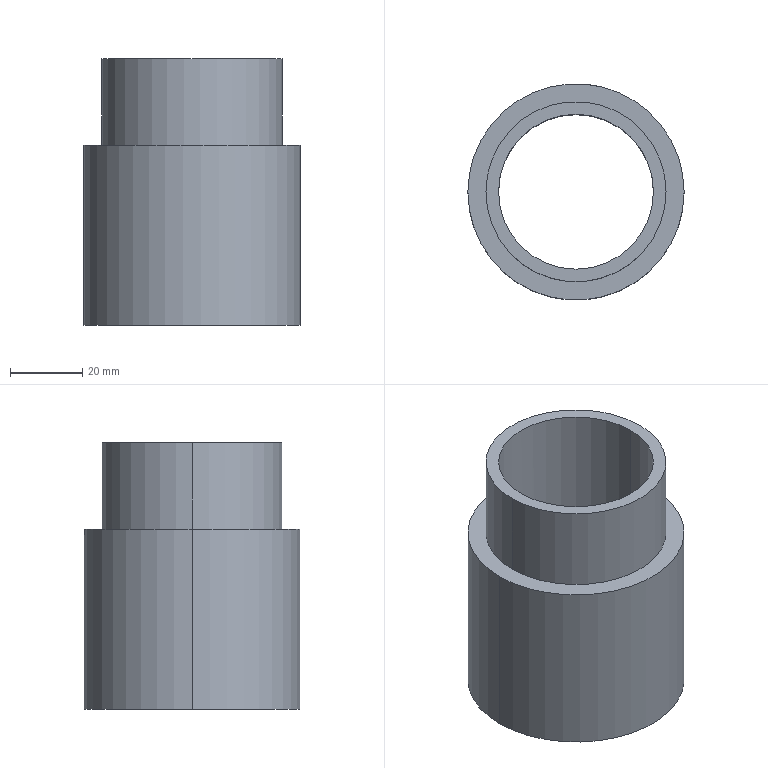Part | SolidWorks | features 3DProfileFeature 1, Extrusion 1, HoleWzd 1, ICE 1 | 1 solid | 11 faces | box 60 x 60 x 74 mm | volume 80866 mm3 | cylinder 8 | plane 3 | commonest cylinder face diameters 5 x2 43 x2 50 x2 60 x2
STEP:
#1=CARTESIAN_POINT('',(25.,0.,24.));
#2=VERTEX_POINT('',#1);
#3=CARTESIAN_POINT('',(-25.,0.,24.));
#4=VERTEX_POINT('',#3);
#5=CARTESIAN_POINT('',(0.,0.,24.));
#6=DIRECTION('',(0.,0.,1.));
#7=DIRECTION('',(1.,0.,0.));
#8=AXIS2_PLACEMENT_3D('',#5,#6,#7);
#9=CIRCLE('',#8,25.);
#10=EDGE_CURVE('',#2,#4,#9,.T.);
#11=ORIENTED_EDGE('',*,*,#10,.F.);
#12=CARTESIAN_POINT('',(25.,0.,0.));
#13=VERTEX_POINT('',#12);
#14=CARTESIAN_POINT('',(25.,0.,24.));
#15=DIRECTION('',(0.,0.,-1.));
#16=VECTOR('',#15,1000.);
#17=LINE('',#14,#16);
#18=EDGE_CURVE('',#2,#13,#17,.T.);
#19=ORIENTED_EDGE('',*,*,#18,.T.);
#20=CARTESIAN_POINT('',(-25.,0.,0.));
#21=VERTEX_POINT('',#20);
#22=CARTESIAN_POINT('',(0.,0.,0.));
#23=DIRECTION('',(0.,0.,1.));
#24=DIRECTION('',(1.,0.,0.));
#25=AXIS2_PLACEMENT_3D('',#22,#23,#24);
#26=CIRCLE('',#25,25.);
#27=EDGE_CURVE('',#13,#21,#26,.T.);
#28=ORIENTED_EDGE('',*,*,#27,.T.);
#29=CARTESIAN_POINT('',(-25.,0.,24.));
#30=DIRECTION('',(0.,0.,-1.));
#31=VECTOR('',#30,1000.);
#32=LINE('',#29,#31);
#33=EDGE_CURVE('',#4,#21,#32,.T.);
#34=ORIENTED_EDGE('',*,*,#33,.F.);
#35=EDGE_LOOP('',(#11,#19,#28,#34));
#36=FACE_OUTER_BOUND('',#35,.T.);
#37=CARTESIAN_POINT('',(0.,0.,24.));
#38=DIRECTION('',(0.,0.,-1.));
#39=DIRECTION('',(-1.,0.,0.));
#40=AXIS2_PLACEMENT_3D('',#37,#38,#39);
#41=CYLINDRICAL_SURFACE('',#40,25.);
#42=ADVANCED_FACE('',(#36),#41,.T.);
#43=CARTESIAN_POINT('',(4.954,20.921,-40.));
#44=VERTEX_POINT('',#43);
#45=CARTESIAN_POINT('',(-0.01248,21.5,-40.));
#46=VERTEX_POINT('',#45);
#47=CARTESIAN_POINT('',(4.954,20.921,-40.));
#48=CARTESIAN_POINT('',(4.954,20.921,-40.163));
#49=CARTESIAN_POINT('',(4.938,20.925,-40.325));
#50=CARTESIAN_POINT('',(4.876,20.94,-40.648));
#51=CARTESIAN_POINT('',(4.829,20.951,-40.806));
#52=CARTESIAN_POINT('',(4.706,20.979,-41.107));
#53=CARTESIAN_POINT('',(4.63,20.996,-41.252));
#54=CARTESIAN_POINT('',(4.451,21.034,-41.525));
#55=CARTESIAN_POINT('',(4.35,21.056,-41.651));
#56=CARTESIAN_POINT('',(4.123,21.101,-41.882));
#57=CARTESIAN_POINT('',(3.996,21.126,-41.987));
#58=CARTESIAN_POINT('',(3.729,21.175,-42.169));
#59=CARTESIAN_POINT('',(3.587,21.199,-42.246));
#60=CARTESIAN_POINT('',(3.288,21.248,-42.372));
#61=CARTESIAN_POINT('',(3.131,21.271,-42.42));
#62=CARTESIAN_POINT('',(2.815,21.316,-42.484));
#63=CARTESIAN_POINT('',(2.654,21.336,-42.5));
#64=CARTESIAN_POINT('',(2.325,21.375,-42.5));
#65=CARTESIAN_POINT('',(2.164,21.391,-42.484));
#66=CARTESIAN_POINT('',(1.845,21.421,-42.421));
#67=CARTESIAN_POINT('',(1.687,21.434,-42.373));
#68=CARTESIAN_POINT('',(1.384,21.456,-42.247));
#69=CARTESIAN_POINT('',(1.241,21.465,-42.171));
#70=CARTESIAN_POINT('',(0.9689,21.479,-41.989));
#71=CARTESIAN_POINT('',(0.8401,21.484,-41.884));
#72=CARTESIAN_POINT('',(0.6089,21.492,-41.654));
#73=CARTESIAN_POINT('',(0.505,21.494,-41.528));
#74=CARTESIAN_POINT('',(0.3212,21.498,-41.255));
#75=CARTESIAN_POINT('',(0.2431,21.499,-41.11));
#76=CARTESIAN_POINT('',(0.05455,21.5,-40.659));
#77=CARTESIAN_POINT('',(-0.01248,21.5,-40.331));
#78=CARTESIAN_POINT('',(-0.01248,21.5,-40.));
#79=B_SPLINE_CURVE_WITH_KNOTS('',3,(#47,#48,#49,#50,#51,#52,#53,#54,#55,#56,#57,#58,#59,#60,#61,#62,#63,#64,#65,#66,#67,#68,#69,#70,#71,#72,#73,#74,#75,#76,#77,#78),.UNSPECIFIED.,.F.,.F.,(4,2,2,2,2,2,2,2,2,2,2,2,2,2,2,4),(0.007823,0.008312,0.0088,0.009289,0.009778,0.01027,0.01076,0.01124,0.01173,0.01222,0.01271,0.0132,0.01369,0.01418,0.01467,0.01564),.UNSPECIFIED.);
#80=EDGE_CURVE('',#44,#46,#79,.T.);
#81=ORIENTED_EDGE('',*,*,#80,.F.);
#82=CARTESIAN_POINT('',(5.942,29.406,-40.));
#83=VERTEX_POINT('',#82);
#84=CARTESIAN_POINT('',(5.954,29.509,-40.));
#85=DIRECTION('',(0.1157,0.9933,0.));
#86=VECTOR('',#85,1000.);
#87=LINE('',#84,#86);
#88=EDGE_CURVE('',#44,#83,#87,.T.);
#89=ORIENTED_EDGE('',*,*,#88,.T.);
#90=CARTESIAN_POINT('',(0.9758,29.984,-40.));
#91=VERTEX_POINT('',#90);
#92=CARTESIAN_POINT('',(5.942,29.406,-40.));
#93=CARTESIAN_POINT('',(5.942,29.406,-40.163));
#94=CARTESIAN_POINT('',(5.927,29.409,-40.325));
#95=CARTESIAN_POINT('',(5.864,29.421,-40.648));
#96=CARTESIAN_POINT('',(5.816,29.431,-40.806));
#97=CARTESIAN_POINT('',(5.694,29.455,-41.107));
#98=CARTESIAN_POINT('',(5.618,29.469,-41.252));
#99=CARTESIAN_POINT('',(5.438,29.503,-41.525));
#100=CARTESIAN_POINT('',(5.336,29.522,-41.651));
#101=CARTESIAN_POINT('',(5.109,29.562,-41.882));
#102=CARTESIAN_POINT('',(4.982,29.584,-41.987));
#103=CARTESIAN_POINT('',(4.713,29.628,-42.169));
#104=CARTESIAN_POINT('',(4.572,29.65,-42.246));
#105=CARTESIAN_POINT('',(4.272,29.695,-42.372));
#106=CARTESIAN_POINT('',(4.115,29.717,-42.42));
#107=CARTESIAN_POINT('',(3.798,29.759,-42.484));
#108=CARTESIAN_POINT('',(3.637,29.779,-42.5));
#109=CARTESIAN_POINT('',(3.309,29.817,-42.5));
#110=CARTESIAN_POINT('',(3.147,29.835,-42.484));
#111=CARTESIAN_POINT('',(2.829,29.867,-42.421));
#112=CARTESIAN_POINT('',(2.671,29.881,-42.373));
#113=CARTESIAN_POINT('',(2.369,29.907,-42.247));
#114=CARTESIAN_POINT('',(2.226,29.918,-42.171));
#115=CARTESIAN_POINT('',(1.954,29.937,-41.99));
#116=CARTESIAN_POINT('',(1.826,29.945,-41.884));
#117=CARTESIAN_POINT('',(1.595,29.958,-41.654));
#118=CARTESIAN_POINT('',(1.491,29.963,-41.528));
#119=CARTESIAN_POINT('',(1.308,29.972,-41.255));
#120=CARTESIAN_POINT('',(1.23,29.975,-41.11));
#121=CARTESIAN_POINT('',(1.042,29.982,-40.659));
#122=CARTESIAN_POINT('',(0.9758,29.984,-40.33));
#123=CARTESIAN_POINT('',(0.9758,29.984,-40.));
#124=B_SPLINE_CURVE_WITH_KNOTS('',3,(#92,#93,#94,#95,#96,#97,#98,#99,#100,#101,#102,#103,#104,#105,#106,#107,#108,#109,#110,#111,#112,#113,#114,#115,#116,#117,#118,#119,#120,#121,#122,#123),.UNSPECIFIED.,.F.,.F.,(4,2,2,2,2,2,2,2,2,2,2,2,2,2,2,4),(0.00782,0.008308,0.008797,0.009285,0.009774,0.01026,0.01075,0.01124,0.01173,0.01222,0.01271,0.01319,0.01368,0.01417,0.01466,0.01564),.UNSPECIFIED.);
#125=EDGE_CURVE('',#83,#91,#124,.T.);
#126=ORIENTED_EDGE('',*,*,#125,.T.);
#127=CARTESIAN_POINT('',(0.9879,30.088,-40.));
#128=DIRECTION('',(0.1157,0.9933,0.));
#129=VECTOR('',#128,1000.);
#130=LINE('',#127,#129);
#131=EDGE_CURVE('',#46,#91,#130,.T.);
#132=ORIENTED_EDGE('',*,*,#131,.F.);
#133=EDGE_LOOP('',(#81,#89,#126,#132));
#134=FACE_OUTER_BOUND('',#133,.T.);
#135=CARTESIAN_POINT('',(3.471,29.799,-40.));
#136=DIRECTION('',(0.1157,0.9933,0.));
#137=DIRECTION('',(-0.9933,0.1157,0.));
#138=AXIS2_PLACEMENT_3D('',#135,#136,#137);
#139=CYLINDRICAL_SURFACE('',#138,2.5);
#140=ADVANCED_FACE('',(#134),#139,.F.);
#141=CARTESIAN_POINT('',(-21.5,0.,-50.));
#142=VERTEX_POINT('',#141);
#143=CARTESIAN_POINT('',(21.5,0.,-50.));
#144=VERTEX_POINT('',#143);
#145=CARTESIAN_POINT('',(0.,0.,-50.));
#146=DIRECTION('',(0.,0.,1.));
#147=DIRECTION('',(1.,0.,0.));
#148=AXIS2_PLACEMENT_3D('',#145,#146,#147);
#149=CIRCLE('',#148,21.5);
#150=EDGE_CURVE('',#142,#144,#149,.T.);
#151=ORIENTED_EDGE('',*,*,#150,.F.);
#152=CARTESIAN_POINT('',(-21.5,0.,24.));
#153=VERTEX_POINT('',#152);
#154=CARTESIAN_POINT('',(-21.5,0.,-50.));
#155=DIRECTION('',(0.,0.,1.));
#156=VECTOR('',#155,1000.);
#157=LINE('',#154,#156);
#158=EDGE_CURVE('',#142,#153,#157,.T.);
#159=ORIENTED_EDGE('',*,*,#158,.T.);
#160=CARTESIAN_POINT('',(21.5,0.,24.));
#161=VERTEX_POINT('',#160);
#162=CARTESIAN_POINT('',(0.,0.,24.));
#163=DIRECTION('',(0.,0.,1.));
#164=DIRECTION('',(1.,0.,0.));
#165=AXIS2_PLACEMENT_3D('',#162,#163,#164);
#166=CIRCLE('',#165,21.5);
#167=EDGE_CURVE('',#153,#161,#166,.T.);
#168=ORIENTED_EDGE('',*,*,#167,.T.);
#169=CARTESIAN_POINT('',(21.5,0.,-50.));
#170=DIRECTION('',(0.,0.,1.));
#171=VECTOR('',#170,1000.);
#172=LINE('',#169,#171);
#173=EDGE_CURVE('',#144,#161,#172,.T.);
#174=ORIENTED_EDGE('',*,*,#173,.F.);
#175=EDGE_LOOP('',(#151,#159,#168,#174));
#176=FACE_OUTER_BOUND('',#175,.T.);
#177=CARTESIAN_POINT('',(0.,0.,-50.));
#178=DIRECTION('',(0.,0.,1.));
#179=DIRECTION('',(1.,0.,0.));
#180=AXIS2_PLACEMENT_3D('',#177,#178,#179);
#181=CYLINDRICAL_SURFACE('',#180,21.5);
#182=ADVANCED_FACE('',(#176),#181,.F.);
#183=CARTESIAN_POINT('',(0.9758,29.984,-40.));
#184=CARTESIAN_POINT('',(0.9758,29.984,-39.835));
#185=CARTESIAN_POINT('',(0.9921,29.984,-39.672));
#186=CARTESIAN_POINT('',(1.056,29.981,-39.353));
#187=CARTESIAN_POINT('',(1.104,29.98,-39.194));
#188=CARTESIAN_POINT('',(1.23,29.975,-38.891));
#189=CARTESIAN_POINT('',(1.307,29.972,-38.747));
#190=CARTESIAN_POINT('',(1.489,29.963,-38.476));
#191=CARTESIAN_POINT('',(1.594,29.958,-38.347));
#192=CARTESIAN_POINT('',(1.825,29.945,-38.117));
#193=CARTESIAN_POINT('',(1.951,29.937,-38.013));
#194=CARTESIAN_POINT('',(2.223,29.918,-37.83));
#195=CARTESIAN_POINT('',(2.369,29.907,-37.753));
#196=CARTESIAN_POINT('',(2.669,29.881,-37.628));
#197=CARTESIAN_POINT('',(2.826,29.867,-37.58));
#198=CARTESIAN_POINT('',(3.147,29.835,-37.516));
#199=CARTESIAN_POINT('',(3.308,29.817,-37.5));
#200=CARTESIAN_POINT('',(3.632,29.78,-37.5));
#201=CARTESIAN_POINT('',(3.797,29.759,-37.516));
#202=CARTESIAN_POINT('',(4.115,29.717,-37.58));
#203=CARTESIAN_POINT('',(4.269,29.695,-37.627));
#204=CARTESIAN_POINT('',(4.569,29.65,-37.753));
#205=CARTESIAN_POINT('',(4.713,29.628,-37.831));
#206=CARTESIAN_POINT('',(4.981,29.584,-38.012));
#207=CARTESIAN_POINT('',(5.105,29.563,-38.115));
#208=CARTESIAN_POINT('',(5.336,29.522,-38.349));
#209=CARTESIAN_POINT('',(5.438,29.503,-38.475));
#210=CARTESIAN_POINT('',(5.616,29.47,-38.746));
#211=CARTESIAN_POINT('',(5.693,29.455,-38.892));
#212=CARTESIAN_POINT('',(5.817,29.431,-39.195));
#213=CARTESIAN_POINT('',(5.863,29.421,-39.351));
#214=CARTESIAN_POINT('',(5.926,29.409,-39.671));
#215=CARTESIAN_POINT('',(5.942,29.406,-39.837));
#216=CARTESIAN_POINT('',(5.942,29.406,-40.));
#217=B_SPLINE_CURVE_WITH_KNOTS('',3,(#183,#184,#185,#186,#187,#188,#189,#190,#191,#192,#193,#194,#195,#196,#197,#198,#199,#200,#201,#202,#203,#204,#205,#206,#207,#208,#209,#210,#211,#212,#213,#214,#215,#216),.UNSPECIFIED.,.F.,.F.,(4,2,2,2,2,2,2,2,2,2,2,2,2,2,2,2,4),(0.,0.0004887,0.0009774,0.001466,0.001955,0.002444,0.002932,0.003421,0.00391,0.004398,0.004887,0.005376,0.005865,0.006353,0.006842,0.007331,0.00782),.UNSPECIFIED.);
#218=EDGE_CURVE('',#91,#83,#217,.T.);
#219=ORIENTED_EDGE('',*,*,#218,.F.);
#220=ORIENTED_EDGE('',*,*,#125,.F.);
#221=EDGE_LOOP('',(#219,#220));
#222=FACE_BOUND('',#221,.T.);
#223=CARTESIAN_POINT('',(30.,0.,-50.));
#224=VERTEX_POINT('',#223);
#225=CARTESIAN_POINT('',(-30.,0.,-50.));
#226=VERTEX_POINT('',#225);
#227=CARTESIAN_POINT('',(0.,0.,-50.));
#228=DIRECTION('',(0.,0.,1.));
#229=DIRECTION('',(1.,0.,0.));
#230=AXIS2_PLACEMENT_3D('',#227,#228,#229);
#231=CIRCLE('',#230,30.);
#232=EDGE_CURVE('',#224,#226,#231,.T.);
#233=ORIENTED_EDGE('',*,*,#232,.T.);
#234=CARTESIAN_POINT('',(-30.,0.,0.));
#235=VERTEX_POINT('',#234);
#236=CARTESIAN_POINT('',(-30.,0.,-50.));
#237=DIRECTION('',(0.,0.,1.));
#238=VECTOR('',#237,1000.);
#239=LINE('',#236,#238);
#240=EDGE_CURVE('',#226,#235,#239,.T.);
#241=ORIENTED_EDGE('',*,*,#240,.T.);
#242=CARTESIAN_POINT('',(30.,0.,0.));
#243=VERTEX_POINT('',#242);
#244=CARTESIAN_POINT('',(0.,0.,0.));
#245=DIRECTION('',(0.,0.,1.));
#246=DIRECTION('',(1.,0.,0.));
#247=AXIS2_PLACEMENT_3D('',#244,#245,#246);
#248=CIRCLE('',#247,30.);
#249=EDGE_CURVE('',#243,#235,#248,.T.);
#250=ORIENTED_EDGE('',*,*,#249,.F.);
#251=CARTESIAN_POINT('',(30.,0.,-50.));
#252=DIRECTION('',(0.,0.,1.));
#253=VECTOR('',#252,1000.);
#254=LINE('',#251,#253);
#255=EDGE_CURVE('',#224,#243,#254,.T.);
#256=ORIENTED_EDGE('',*,*,#255,.F.);
#257=EDGE_LOOP('',(#233,#241,#250,#256));
#258=FACE_OUTER_BOUND('',#257,.T.);
#259=CARTESIAN_POINT('',(0.,0.,-50.));
#260=DIRECTION('',(0.,0.,1.));
#261=DIRECTION('',(1.,0.,0.));
#262=AXIS2_PLACEMENT_3D('',#259,#260,#261);
#263=CYLINDRICAL_SURFACE('',#262,30.);
#264=ADVANCED_FACE('',(#222,#258),#263,.T.);
#265=ORIENTED_EDGE('',*,*,#249,.T.);
#266=CARTESIAN_POINT('',(0.,0.,0.));
#267=DIRECTION('',(0.,0.,1.));
#268=DIRECTION('',(1.,0.,0.));
#269=AXIS2_PLACEMENT_3D('',#266,#267,#268);
#270=CIRCLE('',#269,30.);
#271=EDGE_CURVE('',#235,#243,#270,.T.);
#272=ORIENTED_EDGE('',*,*,#271,.T.);
#273=EDGE_LOOP('',(#265,#272));
#274=FACE_OUTER_BOUND('',#273,.T.);
#275=CARTESIAN_POINT('',(0.,0.,0.));
#276=DIRECTION('',(0.,0.,1.));
#277=DIRECTION('',(1.,0.,0.));
#278=AXIS2_PLACEMENT_3D('',#275,#276,#277);
#279=CIRCLE('',#278,25.);
#280=EDGE_CURVE('',#21,#13,#279,.T.);
#281=ORIENTED_EDGE('',*,*,#280,.F.);
#282=ORIENTED_EDGE('',*,*,#27,.F.);
#283=EDGE_LOOP('',(#281,#282));
#284=FACE_BOUND('',#283,.T.);
#285=CARTESIAN_POINT('',(0.,0.,0.));
#286=DIRECTION('',(0.,0.,1.));
#287=DIRECTION('',(1.,0.,0.));
#288=AXIS2_PLACEMENT_3D('',#285,#286,#287);
#289=PLANE('',#288);
#290=ADVANCED_FACE('',(#274,#284),#289,.T.);
#291=ORIENTED_EDGE('',*,*,#240,.F.);
#292=CARTESIAN_POINT('',(0.,0.,-50.));
#293=DIRECTION('',(0.,0.,1.));
#294=DIRECTION('',(1.,0.,0.));
#295=AXIS2_PLACEMENT_3D('',#292,#293,#294);
#296=CIRCLE('',#295,30.);
#297=EDGE_CURVE('',#226,#224,#296,.T.);
#298=ORIENTED_EDGE('',*,*,#297,.T.);
#299=ORIENTED_EDGE('',*,*,#255,.T.);
#300=ORIENTED_EDGE('',*,*,#271,.F.);
#301=EDGE_LOOP('',(#291,#298,#299,#300));
#302=FACE_OUTER_BOUND('',#301,.T.);
#303=CARTESIAN_POINT('',(0.,0.,-50.));
#304=DIRECTION('',(0.,0.,1.));
#305=DIRECTION('',(1.,0.,0.));
#306=AXIS2_PLACEMENT_3D('',#303,#304,#305);
#307=CYLINDRICAL_SURFACE('',#306,30.);
#308=ADVANCED_FACE('',(#302),#307,.T.);
#309=CARTESIAN_POINT('',(0.,0.,-50.));
#310=DIRECTION('',(0.,0.,1.));
#311=DIRECTION('',(1.,0.,0.));
#312=AXIS2_PLACEMENT_3D('',#309,#310,#311);
#313=CIRCLE('',#312,21.5);
#314=EDGE_CURVE('',#144,#142,#313,.T.);
#315=ORIENTED_EDGE('',*,*,#314,.T.);
#316=ORIENTED_EDGE('',*,*,#150,.T.);
#317=EDGE_LOOP('',(#315,#316));
#318=FACE_BOUND('',#317,.T.);
#319=ORIENTED_EDGE('',*,*,#232,.F.);
#320=ORIENTED_EDGE('',*,*,#297,.F.);
#321=EDGE_LOOP('',(#319,#320));
#322=FACE_OUTER_BOUND('',#321,.T.);
#323=CARTESIAN_POINT('',(0.,0.,-50.));
#324=DIRECTION('',(0.,0.,1.));
#325=DIRECTION('',(1.,0.,0.));
#326=AXIS2_PLACEMENT_3D('',#323,#324,#325);
#327=PLANE('',#326);
#328=ADVANCED_FACE('',(#318,#322),#327,.F.);
#329=ORIENTED_EDGE('',*,*,#158,.F.);
#330=ORIENTED_EDGE('',*,*,#314,.F.);
#331=ORIENTED_EDGE('',*,*,#173,.T.);
#332=CARTESIAN_POINT('',(0.,0.,24.));
#333=DIRECTION('',(0.,0.,1.));
#334=DIRECTION('',(1.,0.,0.));
#335=AXIS2_PLACEMENT_3D('',#332,#333,#334);
#336=CIRCLE('',#335,21.5);
#337=EDGE_CURVE('',#161,#153,#336,.T.);
#338=ORIENTED_EDGE('',*,*,#337,.T.);
#339=EDGE_LOOP('',(#329,#330,#331,#338));
#340=FACE_OUTER_BOUND('',#339,.T.);
#341=CARTESIAN_POINT('',(-0.01248,21.5,-40.));
#342=CARTESIAN_POINT('',(-0.01248,21.5,-39.835));
#343=CARTESIAN_POINT('',(0.003868,21.5,-39.672));
#344=CARTESIAN_POINT('',(0.06789,21.5,-39.352));
#345=CARTESIAN_POINT('',(0.1163,21.5,-39.194));
#346=CARTESIAN_POINT('',(0.2426,21.499,-38.891));
#347=CARTESIAN_POINT('',(0.3199,21.498,-38.747));
#348=CARTESIAN_POINT('',(0.5021,21.494,-38.476));
#349=CARTESIAN_POINT('',(0.6081,21.492,-38.347));
#350=CARTESIAN_POINT('',(0.8392,21.484,-38.117));
#351=CARTESIAN_POINT('',(0.9652,21.479,-38.013));
#352=CARTESIAN_POINT('',(1.239,21.465,-37.83));
#353=CARTESIAN_POINT('',(1.384,21.456,-37.753));
#354=CARTESIAN_POINT('',(1.684,21.434,-37.628));
#355=CARTESIAN_POINT('',(1.842,21.422,-37.58));
#356=CARTESIAN_POINT('',(2.163,21.392,-37.516));
#357=CARTESIAN_POINT('',(2.325,21.375,-37.5));
#358=CARTESIAN_POINT('',(2.649,21.337,-37.5));
#359=CARTESIAN_POINT('',(2.813,21.316,-37.516));
#360=CARTESIAN_POINT('',(3.131,21.271,-37.58));
#361=CARTESIAN_POINT('',(3.285,21.248,-37.627));
#362=CARTESIAN_POINT('',(3.585,21.2,-37.753));
#363=CARTESIAN_POINT('',(3.729,21.175,-37.831));
#364=CARTESIAN_POINT('',(3.996,21.126,-38.012));
#365=CARTESIAN_POINT('',(4.12,21.102,-38.115));
#366=CARTESIAN_POINT('',(4.35,21.056,-38.349));
#367=CARTESIAN_POINT('',(4.451,21.034,-38.475));
#368=CARTESIAN_POINT('',(4.629,20.996,-38.745));
#369=CARTESIAN_POINT('',(4.706,20.979,-38.892));
#370=CARTESIAN_POINT('',(4.829,20.951,-39.194));
#371=CARTESIAN_POINT('',(4.875,20.94,-39.35));
#372=CARTESIAN_POINT('',(4.938,20.925,-39.671));
#373=CARTESIAN_POINT('',(4.954,20.921,-39.837));
#374=CARTESIAN_POINT('',(4.954,20.921,-40.));
#375=B_SPLINE_CURVE_WITH_KNOTS('',3,(#341,#342,#343,#344,#345,#346,#347,#348,#349,#350,#351,#352,#353,#354,#355,#356,#357,#358,#359,#360,#361,#362,#363,#364,#365,#366,#367,#368,#369,#370,#371,#372,#373,#374),.UNSPECIFIED.,.F.,.F.,(4,2,2,2,2,2,2,2,2,2,2,2,2,2,2,2,4),(0.,0.0004889,0.0009778,0.001467,0.001956,0.002445,0.002934,0.003422,0.003911,0.0044,0.004889,0.005378,0.005867,0.006356,0.006845,0.007334,0.007823),.UNSPECIFIED.);
#376=EDGE_CURVE('',#46,#44,#375,.T.);
#377=ORIENTED_EDGE('',*,*,#376,.T.);
#378=ORIENTED_EDGE('',*,*,#80,.T.);
#379=EDGE_LOOP('',(#377,#378));
#380=FACE_BOUND('',#379,.T.);
#381=CARTESIAN_POINT('',(0.,0.,-50.));
#382=DIRECTION('',(0.,0.,1.));
#383=DIRECTION('',(1.,0.,0.));
#384=AXIS2_PLACEMENT_3D('',#381,#382,#383);
#385=CYLINDRICAL_SURFACE('',#384,21.5);
#386=ADVANCED_FACE('',(#340,#380),#385,.F.);
#387=ORIENTED_EDGE('',*,*,#88,.F.);
#388=ORIENTED_EDGE('',*,*,#376,.F.);
#389=ORIENTED_EDGE('',*,*,#131,.T.);
#390=ORIENTED_EDGE('',*,*,#218,.T.);
#391=EDGE_LOOP('',(#387,#388,#389,#390));
#392=FACE_OUTER_BOUND('',#391,.T.);
#393=CARTESIAN_POINT('',(3.471,29.799,-40.));
#394=DIRECTION('',(0.1157,0.9933,0.));
#395=DIRECTION('',(-0.9933,0.1157,0.));
#396=AXIS2_PLACEMENT_3D('',#393,#394,#395);
#397=CYLINDRICAL_SURFACE('',#396,2.5);
#398=ADVANCED_FACE('',(#392),#397,.F.);
#399=CARTESIAN_POINT('',(0.,0.,24.));
#400=DIRECTION('',(0.,0.,1.));
#401=DIRECTION('',(1.,0.,0.));
#402=AXIS2_PLACEMENT_3D('',#399,#400,#401);
#403=CIRCLE('',#402,25.);
#404=EDGE_CURVE('',#4,#2,#403,.T.);
#405=ORIENTED_EDGE('',*,*,#404,.T.);
#406=ORIENTED_EDGE('',*,*,#10,.T.);
#407=EDGE_LOOP('',(#405,#406));
#408=FACE_OUTER_BOUND('',#407,.T.);
#409=ORIENTED_EDGE('',*,*,#337,.F.);
#410=ORIENTED_EDGE('',*,*,#167,.F.);
#411=EDGE_LOOP('',(#409,#410));
#412=FACE_BOUND('',#411,.T.);
#413=CARTESIAN_POINT('',(0.,0.,24.));
#414=DIRECTION('',(0.,0.,1.));
#415=DIRECTION('',(1.,0.,0.));
#416=AXIS2_PLACEMENT_3D('',#413,#414,#415);
#417=PLANE('',#416);
#418=ADVANCED_FACE('',(#408,#412),#417,.T.);
#419=ORIENTED_EDGE('',*,*,#18,.F.);
#420=ORIENTED_EDGE('',*,*,#404,.F.);
#421=ORIENTED_EDGE('',*,*,#33,.T.);
#422=ORIENTED_EDGE('',*,*,#280,.T.);
#423=EDGE_LOOP('',(#419,#420,#421,#422));
#424=FACE_OUTER_BOUND('',#423,.T.);
#425=CARTESIAN_POINT('',(0.,0.,24.));
#426=DIRECTION('',(0.,0.,-1.));
#427=DIRECTION('',(-1.,0.,0.));
#428=AXIS2_PLACEMENT_3D('',#425,#426,#427);
#429=CYLINDRICAL_SURFACE('',#428,25.);
#430=ADVANCED_FACE('',(#424),#429,.T.);
#431=CLOSED_SHELL('',(#42,#140,#182,#264,#290,#308,#328,#386,#398,#418,#430));
#432=MANIFOLD_SOLID_BREP('',#431);
#433=CARTESIAN_POINT('',(0.,0.,0.));
#434=DIRECTION('',(0.,0.,1.));
#435=DIRECTION('',(1.,0.,0.));
#436=AXIS2_PLACEMENT_3D('',#433,#434,#435);
#437=(LENGTH_UNIT()NAMED_UNIT(*)SI_UNIT(.MILLI.,.METRE.));
#438=UNCERTAINTY_MEASURE_WITH_UNIT(LENGTH_MEASURE(0.00001),#437,'','');
#439=(NAMED_UNIT(*)PLANE_ANGLE_UNIT()SI_UNIT($,.RADIAN.));
#440=(NAMED_UNIT(*)SI_UNIT($,.STERADIAN.)SOLID_ANGLE_UNIT());
#441=(GEOMETRIC_REPRESENTATION_CONTEXT(3)GLOBAL_UNCERTAINTY_ASSIGNED_CONTEXT((#438))GLOBAL_UNIT_ASSIGNED_CONTEXT((#437,#439,#440))REPRESENTATION_CONTEXT('',''));
#442=ADVANCED_BREP_SHAPE_REPRESENTATION('',(#432,#436),#441);